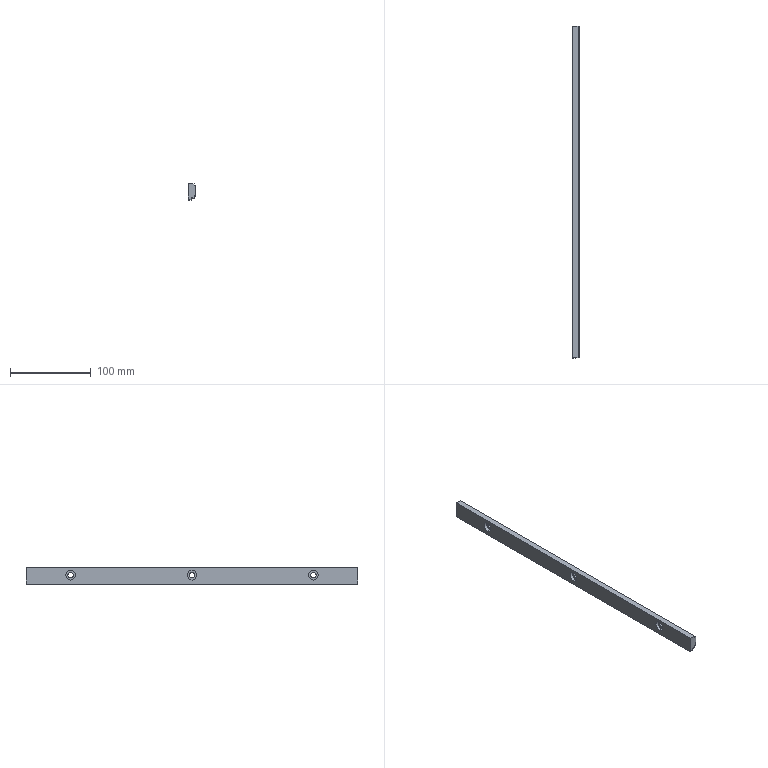Part | STEP file | 1 solid | 33 faces | box 9 x 410 x 20.4 mm | volume 65356 mm3 | cylinder 18 | plane 15 | commonest cylinder face diameters 3 x6 6.5 x6 12 x6